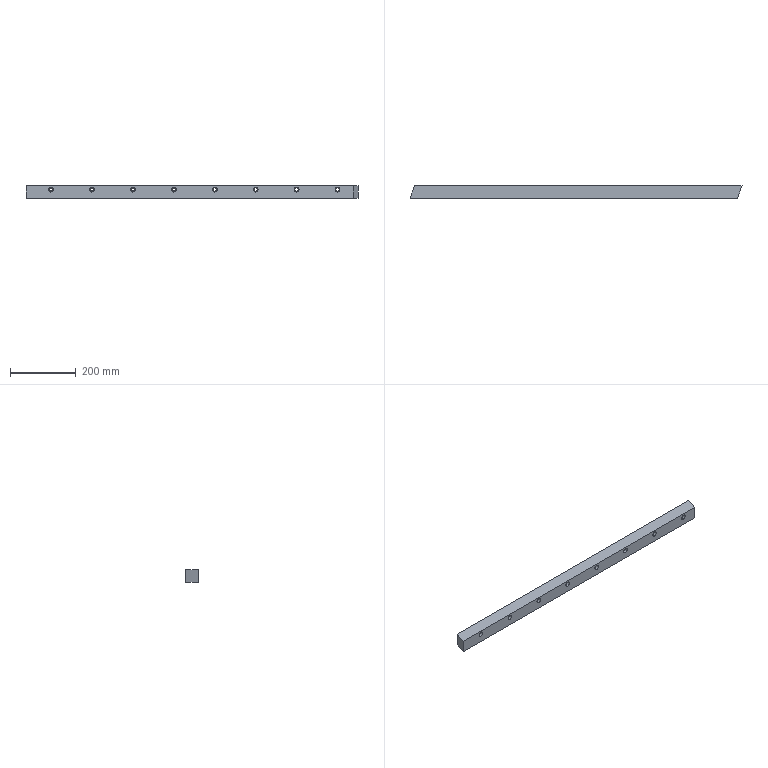Part | STEP file | MHH043910 | 1 solid | 46 faces | box 1014 x 39 x 39 mm | volume 1489427 mm3 | cylinder 32 | plane 14 | commonest cylinder face diameters 10 x16 15 x16
STEP:
#1=CARTESIAN_POINT('',(187.5,-30.,34.5));
#2=VERTEX_POINT('',#1);
#3=CARTESIAN_POINT('',(187.5,-30.,19.5));
#4=VERTEX_POINT('',#3);
#5=CARTESIAN_POINT('',(187.5,-30.,27.));
#6=DIRECTION('',(0.,-1.,0.));
#7=DIRECTION('',(0.,0.,-1.));
#8=AXIS2_PLACEMENT_3D('',#5,#6,#7);
#9=CIRCLE('',#8,7.5);
#10=EDGE_CURVE('',#2,#4,#9,.T.);
#11=ORIENTED_EDGE('',*,*,#10,.F.);
#12=CARTESIAN_POINT('',(187.5,-39.,34.5));
#13=VERTEX_POINT('',#12);
#14=CARTESIAN_POINT('',(187.5,-39.,34.5));
#15=DIRECTION('',(0.,-1.,0.));
#16=VECTOR('',#15,1000.);
#17=LINE('',#14,#16);
#18=EDGE_CURVE('',#2,#13,#17,.T.);
#19=ORIENTED_EDGE('',*,*,#18,.T.);
#20=CARTESIAN_POINT('',(187.5,-39.,19.5));
#21=VERTEX_POINT('',#20);
#22=CARTESIAN_POINT('',(187.5,-39.,27.));
#23=DIRECTION('',(0.,-1.,0.));
#24=DIRECTION('',(0.,0.,-1.));
#25=AXIS2_PLACEMENT_3D('',#22,#23,#24);
#26=CIRCLE('',#25,7.5);
#27=EDGE_CURVE('',#13,#21,#26,.T.);
#28=ORIENTED_EDGE('',*,*,#27,.T.);
#29=CARTESIAN_POINT('',(187.5,-39.,19.5));
#30=DIRECTION('',(0.,-1.,0.));
#31=VECTOR('',#30,1000.);
#32=LINE('',#29,#31);
#33=EDGE_CURVE('',#4,#21,#32,.T.);
#34=ORIENTED_EDGE('',*,*,#33,.F.);
#35=EDGE_LOOP('',(#11,#19,#28,#34));
#36=FACE_OUTER_BOUND('',#35,.T.);
#37=CARTESIAN_POINT('',(187.5,-39.,27.));
#38=DIRECTION('',(0.,-1.,0.));
#39=DIRECTION('',(0.,0.,-1.));
#40=AXIS2_PLACEMENT_3D('',#37,#38,#39);
#41=CYLINDRICAL_SURFACE('',#40,7.5);
#42=ADVANCED_FACE('',(#36),#41,.F.);
#43=CARTESIAN_POINT('',(187.5,0.,32.));
#44=VERTEX_POINT('',#43);
#45=CARTESIAN_POINT('',(187.5,0.,22.));
#46=VERTEX_POINT('',#45);
#47=CARTESIAN_POINT('',(187.5,0.,27.));
#48=DIRECTION('',(0.,-1.,0.));
#49=DIRECTION('',(0.,0.,-1.));
#50=AXIS2_PLACEMENT_3D('',#47,#48,#49);
#51=CIRCLE('',#50,5.);
#52=EDGE_CURVE('',#44,#46,#51,.T.);
#53=ORIENTED_EDGE('',*,*,#52,.F.);
#54=CARTESIAN_POINT('',(187.5,-30.,32.));
#55=VERTEX_POINT('',#54);
#56=CARTESIAN_POINT('',(187.5,-39.,32.));
#57=DIRECTION('',(0.,-1.,0.));
#58=VECTOR('',#57,1000.);
#59=LINE('',#56,#58);
#60=EDGE_CURVE('',#44,#55,#59,.T.);
#61=ORIENTED_EDGE('',*,*,#60,.T.);
#62=CARTESIAN_POINT('',(187.5,-30.,22.));
#63=VERTEX_POINT('',#62);
#64=CARTESIAN_POINT('',(187.5,-30.,27.));
#65=DIRECTION('',(0.,-1.,0.));
#66=DIRECTION('',(0.,0.,-1.));
#67=AXIS2_PLACEMENT_3D('',#64,#65,#66);
#68=CIRCLE('',#67,5.);
#69=EDGE_CURVE('',#55,#63,#68,.T.);
#70=ORIENTED_EDGE('',*,*,#69,.T.);
#71=CARTESIAN_POINT('',(187.5,-39.,22.));
#72=DIRECTION('',(0.,-1.,0.));
#73=VECTOR('',#72,1000.);
#74=LINE('',#71,#73);
#75=EDGE_CURVE('',#46,#63,#74,.T.);
#76=ORIENTED_EDGE('',*,*,#75,.F.);
#77=EDGE_LOOP('',(#53,#61,#70,#76));
#78=FACE_OUTER_BOUND('',#77,.T.);
#79=CARTESIAN_POINT('',(187.5,-39.,27.));
#80=DIRECTION('',(0.,-1.,0.));
#81=DIRECTION('',(0.,0.,-1.));
#82=AXIS2_PLACEMENT_3D('',#79,#80,#81);
#83=CYLINDRICAL_SURFACE('',#82,5.);
#84=ADVANCED_FACE('',(#78),#83,.F.);
#85=CARTESIAN_POINT('',(62.5,-30.,34.5));
#86=VERTEX_POINT('',#85);
#87=CARTESIAN_POINT('',(62.5,-30.,19.5));
#88=VERTEX_POINT('',#87);
#89=CARTESIAN_POINT('',(62.5,-30.,27.));
#90=DIRECTION('',(0.,-1.,0.));
#91=DIRECTION('',(0.,0.,-1.));
#92=AXIS2_PLACEMENT_3D('',#89,#90,#91);
#93=CIRCLE('',#92,7.5);
#94=EDGE_CURVE('',#86,#88,#93,.T.);
#95=ORIENTED_EDGE('',*,*,#94,.F.);
#96=CARTESIAN_POINT('',(62.5,-39.,34.5));
#97=VERTEX_POINT('',#96);
#98=CARTESIAN_POINT('',(62.5,-39.,34.5));
#99=DIRECTION('',(0.,-1.,0.));
#100=VECTOR('',#99,1000.);
#101=LINE('',#98,#100);
#102=EDGE_CURVE('',#86,#97,#101,.T.);
#103=ORIENTED_EDGE('',*,*,#102,.T.);
#104=CARTESIAN_POINT('',(62.5,-39.,19.5));
#105=VERTEX_POINT('',#104);
#106=CARTESIAN_POINT('',(62.5,-39.,27.));
#107=DIRECTION('',(0.,-1.,0.));
#108=DIRECTION('',(0.,0.,-1.));
#109=AXIS2_PLACEMENT_3D('',#106,#107,#108);
#110=CIRCLE('',#109,7.5);
#111=EDGE_CURVE('',#97,#105,#110,.T.);
#112=ORIENTED_EDGE('',*,*,#111,.T.);
#113=CARTESIAN_POINT('',(62.5,-39.,19.5));
#114=DIRECTION('',(0.,-1.,0.));
#115=VECTOR('',#114,1000.);
#116=LINE('',#113,#115);
#117=EDGE_CURVE('',#88,#105,#116,.T.);
#118=ORIENTED_EDGE('',*,*,#117,.F.);
#119=EDGE_LOOP('',(#95,#103,#112,#118));
#120=FACE_OUTER_BOUND('',#119,.T.);
#121=CARTESIAN_POINT('',(62.5,-39.,27.));
#122=DIRECTION('',(0.,-1.,0.));
#123=DIRECTION('',(0.,0.,-1.));
#124=AXIS2_PLACEMENT_3D('',#121,#122,#123);
#125=CYLINDRICAL_SURFACE('',#124,7.5);
#126=ADVANCED_FACE('',(#120),#125,.F.);
#127=CARTESIAN_POINT('',(62.5,0.,32.));
#128=VERTEX_POINT('',#127);
#129=CARTESIAN_POINT('',(62.5,0.,22.));
#130=VERTEX_POINT('',#129);
#131=CARTESIAN_POINT('',(62.5,0.,27.));
#132=DIRECTION('',(0.,-1.,0.));
#133=DIRECTION('',(0.,0.,-1.));
#134=AXIS2_PLACEMENT_3D('',#131,#132,#133);
#135=CIRCLE('',#134,5.);
#136=EDGE_CURVE('',#128,#130,#135,.T.);
#137=ORIENTED_EDGE('',*,*,#136,.F.);
#138=CARTESIAN_POINT('',(62.5,-30.,32.));
#139=VERTEX_POINT('',#138);
#140=CARTESIAN_POINT('',(62.5,-39.,32.));
#141=DIRECTION('',(0.,-1.,0.));
#142=VECTOR('',#141,1000.);
#143=LINE('',#140,#142);
#144=EDGE_CURVE('',#128,#139,#143,.T.);
#145=ORIENTED_EDGE('',*,*,#144,.T.);
#146=CARTESIAN_POINT('',(62.5,-30.,22.));
#147=VERTEX_POINT('',#146);
#148=CARTESIAN_POINT('',(62.5,-30.,27.));
#149=DIRECTION('',(0.,-1.,0.));
#150=DIRECTION('',(0.,0.,-1.));
#151=AXIS2_PLACEMENT_3D('',#148,#149,#150);
#152=CIRCLE('',#151,5.);
#153=EDGE_CURVE('',#139,#147,#152,.T.);
#154=ORIENTED_EDGE('',*,*,#153,.T.);
#155=CARTESIAN_POINT('',(62.5,-39.,22.));
#156=DIRECTION('',(0.,-1.,0.));
#157=VECTOR('',#156,1000.);
#158=LINE('',#155,#157);
#159=EDGE_CURVE('',#130,#147,#158,.T.);
#160=ORIENTED_EDGE('',*,*,#159,.F.);
#161=EDGE_LOOP('',(#137,#145,#154,#160));
#162=FACE_OUTER_BOUND('',#161,.T.);
#163=CARTESIAN_POINT('',(62.5,-39.,27.));
#164=DIRECTION('',(0.,-1.,0.));
#165=DIRECTION('',(0.,0.,-1.));
#166=AXIS2_PLACEMENT_3D('',#163,#164,#165);
#167=CYLINDRICAL_SURFACE('',#166,5.);
#168=ADVANCED_FACE('',(#162),#167,.F.);
#169=CARTESIAN_POINT('',(312.5,0.,32.));
#170=VERTEX_POINT('',#169);
#171=CARTESIAN_POINT('',(312.5,0.,22.));
#172=VERTEX_POINT('',#171);
#173=CARTESIAN_POINT('',(312.5,0.,27.));
#174=DIRECTION('',(0.,-1.,0.));
#175=DIRECTION('',(0.,0.,-1.));
#176=AXIS2_PLACEMENT_3D('',#173,#174,#175);
#177=CIRCLE('',#176,5.);
#178=EDGE_CURVE('',#170,#172,#177,.T.);
#179=ORIENTED_EDGE('',*,*,#178,.F.);
#180=CARTESIAN_POINT('',(312.5,-30.,32.));
#181=VERTEX_POINT('',#180);
#182=CARTESIAN_POINT('',(312.5,-39.,32.));
#183=DIRECTION('',(0.,-1.,0.));
#184=VECTOR('',#183,1000.);
#185=LINE('',#182,#184);
#186=EDGE_CURVE('',#170,#181,#185,.T.);
#187=ORIENTED_EDGE('',*,*,#186,.T.);
#188=CARTESIAN_POINT('',(312.5,-30.,22.));
#189=VERTEX_POINT('',#188);
#190=CARTESIAN_POINT('',(312.5,-30.,27.));
#191=DIRECTION('',(0.,-1.,0.));
#192=DIRECTION('',(0.,0.,-1.));
#193=AXIS2_PLACEMENT_3D('',#190,#191,#192);
#194=CIRCLE('',#193,5.);
#195=EDGE_CURVE('',#181,#189,#194,.T.);
#196=ORIENTED_EDGE('',*,*,#195,.T.);
#197=CARTESIAN_POINT('',(312.5,-39.,22.));
#198=DIRECTION('',(0.,-1.,0.));
#199=VECTOR('',#198,1000.);
#200=LINE('',#197,#199);
#201=EDGE_CURVE('',#172,#189,#200,.T.);
#202=ORIENTED_EDGE('',*,*,#201,.F.);
#203=EDGE_LOOP('',(#179,#187,#196,#202));
#204=FACE_OUTER_BOUND('',#203,.T.);
#205=CARTESIAN_POINT('',(312.5,-39.,27.));
#206=DIRECTION('',(0.,-1.,0.));
#207=DIRECTION('',(0.,0.,-1.));
#208=AXIS2_PLACEMENT_3D('',#205,#206,#207);
#209=CYLINDRICAL_SURFACE('',#208,5.);
#210=ADVANCED_FACE('',(#204),#209,.F.);
#211=CARTESIAN_POINT('',(312.5,-30.,34.5));
#212=VERTEX_POINT('',#211);
#213=CARTESIAN_POINT('',(312.5,-30.,19.5));
#214=VERTEX_POINT('',#213);
#215=CARTESIAN_POINT('',(312.5,-30.,27.));
#216=DIRECTION('',(0.,-1.,0.));
#217=DIRECTION('',(0.,0.,-1.));
#218=AXIS2_PLACEMENT_3D('',#215,#216,#217);
#219=CIRCLE('',#218,7.5);
#220=EDGE_CURVE('',#212,#214,#219,.T.);
#221=ORIENTED_EDGE('',*,*,#220,.F.);
#222=CARTESIAN_POINT('',(312.5,-39.,34.5));
#223=VERTEX_POINT('',#222);
#224=CARTESIAN_POINT('',(312.5,-39.,34.5));
#225=DIRECTION('',(0.,-1.,0.));
#226=VECTOR('',#225,1000.);
#227=LINE('',#224,#226);
#228=EDGE_CURVE('',#212,#223,#227,.T.);
#229=ORIENTED_EDGE('',*,*,#228,.T.);
#230=CARTESIAN_POINT('',(312.5,-39.,19.5));
#231=VERTEX_POINT('',#230);
#232=CARTESIAN_POINT('',(312.5,-39.,27.));
#233=DIRECTION('',(0.,-1.,0.));
#234=DIRECTION('',(0.,0.,-1.));
#235=AXIS2_PLACEMENT_3D('',#232,#233,#234);
#236=CIRCLE('',#235,7.5);
#237=EDGE_CURVE('',#223,#231,#236,.T.);
#238=ORIENTED_EDGE('',*,*,#237,.T.);
#239=CARTESIAN_POINT('',(312.5,-39.,19.5));
#240=DIRECTION('',(0.,-1.,0.));
#241=VECTOR('',#240,1000.);
#242=LINE('',#239,#241);
#243=EDGE_CURVE('',#214,#231,#242,.T.);
#244=ORIENTED_EDGE('',*,*,#243,.F.);
#245=EDGE_LOOP('',(#221,#229,#238,#244));
#246=FACE_OUTER_BOUND('',#245,.T.);
#247=CARTESIAN_POINT('',(312.5,-39.,27.));
#248=DIRECTION('',(0.,-1.,0.));
#249=DIRECTION('',(0.,0.,-1.));
#250=AXIS2_PLACEMENT_3D('',#247,#248,#249);
#251=CYLINDRICAL_SURFACE('',#250,7.5);
#252=ADVANCED_FACE('',(#246),#251,.F.);
#253=CARTESIAN_POINT('',(437.5,0.,32.));
#254=VERTEX_POINT('',#253);
#255=CARTESIAN_POINT('',(437.5,0.,22.));
#256=VERTEX_POINT('',#255);
#257=CARTESIAN_POINT('',(437.5,0.,27.));
#258=DIRECTION('',(0.,-1.,0.));
#259=DIRECTION('',(0.,0.,-1.));
#260=AXIS2_PLACEMENT_3D('',#257,#258,#259);
#261=CIRCLE('',#260,5.);
#262=EDGE_CURVE('',#254,#256,#261,.T.);
#263=ORIENTED_EDGE('',*,*,#262,.F.);
#264=CARTESIAN_POINT('',(437.5,-30.,32.));
#265=VERTEX_POINT('',#264);
#266=CARTESIAN_POINT('',(437.5,-39.,32.));
#267=DIRECTION('',(0.,-1.,0.));
#268=VECTOR('',#267,1000.);
#269=LINE('',#266,#268);
#270=EDGE_CURVE('',#254,#265,#269,.T.);
#271=ORIENTED_EDGE('',*,*,#270,.T.);
#272=CARTESIAN_POINT('',(437.5,-30.,22.));
#273=VERTEX_POINT('',#272);
#274=CARTESIAN_POINT('',(437.5,-30.,27.));
#275=DIRECTION('',(0.,-1.,0.));
#276=DIRECTION('',(0.,0.,-1.));
#277=AXIS2_PLACEMENT_3D('',#274,#275,#276);
#278=CIRCLE('',#277,5.);
#279=EDGE_CURVE('',#265,#273,#278,.T.);
#280=ORIENTED_EDGE('',*,*,#279,.T.);
#281=CARTESIAN_POINT('',(437.5,-39.,22.));
#282=DIRECTION('',(0.,-1.,0.));
#283=VECTOR('',#282,1000.);
#284=LINE('',#281,#283);
#285=EDGE_CURVE('',#256,#273,#284,.T.);
#286=ORIENTED_EDGE('',*,*,#285,.F.);
#287=EDGE_LOOP('',(#263,#271,#280,#286));
#288=FACE_OUTER_BOUND('',#287,.T.);
#289=CARTESIAN_POINT('',(437.5,-39.,27.));
#290=DIRECTION('',(0.,-1.,0.));
#291=DIRECTION('',(0.,0.,-1.));
#292=AXIS2_PLACEMENT_3D('',#289,#290,#291);
#293=CYLINDRICAL_SURFACE('',#292,5.);
#294=ADVANCED_FACE('',(#288),#293,.F.);
#295=CARTESIAN_POINT('',(437.5,-30.,34.5));
#296=VERTEX_POINT('',#295);
#297=CARTESIAN_POINT('',(437.5,-30.,19.5));
#298=VERTEX_POINT('',#297);
#299=CARTESIAN_POINT('',(437.5,-30.,27.));
#300=DIRECTION('',(0.,-1.,0.));
#301=DIRECTION('',(0.,0.,-1.));
#302=AXIS2_PLACEMENT_3D('',#299,#300,#301);
#303=CIRCLE('',#302,7.5);
#304=EDGE_CURVE('',#296,#298,#303,.T.);
#305=ORIENTED_EDGE('',*,*,#304,.F.);
#306=CARTESIAN_POINT('',(437.5,-39.,34.5));
#307=VERTEX_POINT('',#306);
#308=CARTESIAN_POINT('',(437.5,-39.,34.5));
#309=DIRECTION('',(0.,-1.,0.));
#310=VECTOR('',#309,1000.);
#311=LINE('',#308,#310);
#312=EDGE_CURVE('',#296,#307,#311,.T.);
#313=ORIENTED_EDGE('',*,*,#312,.T.);
#314=CARTESIAN_POINT('',(437.5,-39.,19.5));
#315=VERTEX_POINT('',#314);
#316=CARTESIAN_POINT('',(437.5,-39.,27.));
#317=DIRECTION('',(0.,-1.,0.));
#318=DIRECTION('',(0.,0.,-1.));
#319=AXIS2_PLACEMENT_3D('',#316,#317,#318);
#320=CIRCLE('',#319,7.5);
#321=EDGE_CURVE('',#307,#315,#320,.T.);
#322=ORIENTED_EDGE('',*,*,#321,.T.);
#323=CARTESIAN_POINT('',(437.5,-39.,19.5));
#324=DIRECTION('',(0.,-1.,0.));
#325=VECTOR('',#324,1000.);
#326=LINE('',#323,#325);
#327=EDGE_CURVE('',#298,#315,#326,.T.);
#328=ORIENTED_EDGE('',*,*,#327,.F.);
#329=EDGE_LOOP('',(#305,#313,#322,#328));
#330=FACE_OUTER_BOUND('',#329,.T.);
#331=CARTESIAN_POINT('',(437.5,-39.,27.));
#332=DIRECTION('',(0.,-1.,0.));
#333=DIRECTION('',(0.,0.,-1.));
#334=AXIS2_PLACEMENT_3D('',#331,#332,#333);
#335=CYLINDRICAL_SURFACE('',#334,7.5);
#336=ADVANCED_FACE('',(#330),#335,.F.);
#337=CARTESIAN_POINT('',(562.5,0.,32.));
#338=VERTEX_POINT('',#337);
#339=CARTESIAN_POINT('',(562.5,0.,22.));
#340=VERTEX_POINT('',#339);
#341=CARTESIAN_POINT('',(562.5,0.,27.));
#342=DIRECTION('',(0.,-1.,0.));
#343=DIRECTION('',(0.,0.,-1.));
#344=AXIS2_PLACEMENT_3D('',#341,#342,#343);
#345=CIRCLE('',#344,5.);
#346=EDGE_CURVE('',#338,#340,#345,.T.);
#347=ORIENTED_EDGE('',*,*,#346,.F.);
#348=CARTESIAN_POINT('',(562.5,-30.,32.));
#349=VERTEX_POINT('',#348);
#350=CARTESIAN_POINT('',(562.5,-39.,32.));
#351=DIRECTION('',(0.,-1.,0.));
#352=VECTOR('',#351,1000.);
#353=LINE('',#350,#352);
#354=EDGE_CURVE('',#338,#349,#353,.T.);
#355=ORIENTED_EDGE('',*,*,#354,.T.);
#356=CARTESIAN_POINT('',(562.5,-30.,22.));
#357=VERTEX_POINT('',#356);
#358=CARTESIAN_POINT('',(562.5,-30.,27.));
#359=DIRECTION('',(0.,-1.,0.));
#360=DIRECTION('',(0.,0.,-1.));
#361=AXIS2_PLACEMENT_3D('',#358,#359,#360);
#362=CIRCLE('',#361,5.);
#363=EDGE_CURVE('',#349,#357,#362,.T.);
#364=ORIENTED_EDGE('',*,*,#363,.T.);
#365=CARTESIAN_POINT('',(562.5,-39.,22.));
#366=DIRECTION('',(0.,-1.,0.));
#367=VECTOR('',#366,1000.);
#368=LINE('',#365,#367);
#369=EDGE_CURVE('',#340,#357,#368,.T.);
#370=ORIENTED_EDGE('',*,*,#369,.F.);
#371=EDGE_LOOP('',(#347,#355,#364,#370));
#372=FACE_OUTER_BOUND('',#371,.T.);
#373=CARTESIAN_POINT('',(562.5,-39.,27.));
#374=DIRECTION('',(0.,-1.,0.));
#375=DIRECTION('',(0.,0.,-1.));
#376=AXIS2_PLACEMENT_3D('',#373,#374,#375);
#377=CYLINDRICAL_SURFACE('',#376,5.);
#378=ADVANCED_FACE('',(#372),#377,.F.);
#379=CARTESIAN_POINT('',(562.5,-30.,34.5));
#380=VERTEX_POINT('',#379);
#381=CARTESIAN_POINT('',(562.5,-30.,19.5));
#382=VERTEX_POINT('',#381);
#383=CARTESIAN_POINT('',(562.5,-30.,27.));
#384=DIRECTION('',(0.,-1.,0.));
#385=DIRECTION('',(0.,0.,-1.));
#386=AXIS2_PLACEMENT_3D('',#383,#384,#385);
#387=CIRCLE('',#386,7.5);
#388=EDGE_CURVE('',#380,#382,#387,.T.);
#389=ORIENTED_EDGE('',*,*,#388,.F.);
#390=CARTESIAN_POINT('',(562.5,-39.,34.5));
#391=VERTEX_POINT('',#390);
#392=CARTESIAN_POINT('',(562.5,-39.,34.5));
#393=DIRECTION('',(0.,-1.,0.));
#394=VECTOR('',#393,1000.);
#395=LINE('',#392,#394);
#396=EDGE_CURVE('',#380,#391,#395,.T.);
#397=ORIENTED_EDGE('',*,*,#396,.T.);
#398=CARTESIAN_POINT('',(562.5,-39.,19.5));
#399=VERTEX_POINT('',#398);
#400=CARTESIAN_POINT('',(562.5,-39.,27.));
#401=DIRECTION('',(0.,-1.,0.));
#402=DIRECTION('',(0.,0.,-1.));
#403=AXIS2_PLACEMENT_3D('',#400,#401,#402);
#404=CIRCLE('',#403,7.5);
#405=EDGE_CURVE('',#391,#399,#404,.T.);
#406=ORIENTED_EDGE('',*,*,#405,.T.);
#407=CARTESIAN_POINT('',(562.5,-39.,19.5));
#408=DIRECTION('',(0.,-1.,0.));
#409=VECTOR('',#408,1000.);
#410=LINE('',#407,#409);
#411=EDGE_CURVE('',#382,#399,#410,.T.);
#412=ORIENTED_EDGE('',*,*,#411,.F.);
#413=EDGE_LOOP('',(#389,#397,#406,#412));
#414=FACE_OUTER_BOUND('',#413,.T.);
#415=CARTESIAN_POINT('',(562.5,-39.,27.));
#416=DIRECTION('',(0.,-1.,0.));
#417=DIRECTION('',(0.,0.,-1.));
#418=AXIS2_PLACEMENT_3D('',#415,#416,#417);
#419=CYLINDRICAL_SURFACE('',#418,7.5);
#420=ADVANCED_FACE('',(#414),#419,.F.);
#421=CARTESIAN_POINT('',(687.5,0.,32.));
#422=VERTEX_POINT('',#421);
#423=CARTESIAN_POINT('',(687.5,0.,22.));
#424=VERTEX_POINT('',#423);
#425=CARTESIAN_POINT('',(687.5,0.,27.));
#426=DIRECTION('',(0.,-1.,0.));
#427=DIRECTION('',(0.,0.,-1.));
#428=AXIS2_PLACEMENT_3D('',#425,#426,#427);
#429=CIRCLE('',#428,5.);
#430=EDGE_CURVE('',#422,#424,#429,.T.);
#431=ORIENTED_EDGE('',*,*,#430,.F.);
#432=CARTESIAN_POINT('',(687.5,-30.,32.));
#433=VERTEX_POINT('',#432);
#434=CARTESIAN_POINT('',(687.5,-39.,32.));
#435=DIRECTION('',(0.,-1.,0.));
#436=VECTOR('',#435,1000.);
#437=LINE('',#434,#436);
#438=EDGE_CURVE('',#422,#433,#437,.T.);
#439=ORIENTED_EDGE('',*,*,#438,.T.);
#440=CARTESIAN_POINT('',(687.5,-30.,22.));
#441=VERTEX_POINT('',#440);
#442=CARTESIAN_POINT('',(687.5,-30.,27.));
#443=DIRECTION('',(0.,-1.,0.));
#444=DIRECTION('',(0.,0.,-1.));
#445=AXIS2_PLACEMENT_3D('',#442,#443,#444);
#446=CIRCLE('',#445,5.);
#447=EDGE_CURVE('',#433,#441,#446,.T.);
#448=ORIENTED_EDGE('',*,*,#447,.T.);
#449=CARTESIAN_POINT('',(687.5,-39.,22.));
#450=DIRECTION('',(0.,-1.,0.));
#451=VECTOR('',#450,1000.);
#452=LINE('',#449,#451);
#453=EDGE_CURVE('',#424,#441,#452,.T.);
#454=ORIENTED_EDGE('',*,*,#453,.F.);
#455=EDGE_LOOP('',(#431,#439,#448,#454));
#456=FACE_OUTER_BOUND('',#455,.T.);
#457=CARTESIAN_POINT('',(687.5,-39.,27.));
#458=DIRECTION('',(0.,-1.,0.));
#459=DIRECTION('',(0.,0.,-1.));
#460=AXIS2_PLACEMENT_3D('',#457,#458,#459);
#461=CYLINDRICAL_SURFACE('',#460,5.);
#462=ADVANCED_FACE('',(#456),#461,.F.);
#463=CARTESIAN_POINT('',(687.5,-30.,34.5));
#464=VERTEX_POINT('',#463);
#465=CARTESIAN_POINT('',(687.5,-30.,19.5));
#466=VERTEX_POINT('',#465);
#467=CARTESIAN_POINT('',(687.5,-30.,27.));
#468=DIRECTION('',(0.,-1.,0.));
#469=DIRECTION('',(0.,0.,-1.));
#470=AXIS2_PLACEMENT_3D('',#467,#468,#469);
#471=CIRCLE('',#470,7.5);
#472=EDGE_CURVE('',#464,#466,#471,.T.);
#473=ORIENTED_EDGE('',*,*,#472,.F.);
#474=CARTESIAN_POINT('',(687.5,-39.,34.5));
#475=VERTEX_POINT('',#474);
#476=CARTESIAN_POINT('',(687.5,-39.,34.5));
#477=DIRECTION('',(0.,-1.,0.));
#478=VECTOR('',#477,1000.);
#479=LINE('',#476,#478);
#480=EDGE_CURVE('',#464,#475,#479,.T.);
#481=ORIENTED_EDGE('',*,*,#480,.T.);
#482=CARTESIAN_POINT('',(687.5,-39.,19.5));
#483=VERTEX_POINT('',#482);
#484=CARTESIAN_POINT('',(687.5,-39.,27.));
#485=DIRECTION('',(0.,-1.,0.));
#486=DIRECTION('',(0.,0.,-1.));
#487=AXIS2_PLACEMENT_3D('',#484,#485,#486);
#488=CIRCLE('',#487,7.5);
#489=EDGE_CURVE('',#475,#483,#488,.T.);
#490=ORIENTED_EDGE('',*,*,#489,.T.);
#491=CARTESIAN_POINT('',(687.5,-39.,19.5));
#492=DIRECTION('',(0.,-1.,0.));
#493=VECTOR('',#492,1000.);
#494=LINE('',#491,#493);
#495=EDGE_CURVE('',#466,#483,#494,.T.);
#496=ORIENTED_EDGE('',*,*,#495,.F.);
#497=EDGE_LOOP('',(#473,#481,#490,#496));
#498=FACE_OUTER_BOUND('',#497,.T.);
#499=CARTESIAN_POINT('',(687.5,-39.,27.));
#500=DIRECTION('',(0.,-1.,0.));
#501=DIRECTION('',(0.,0.,-1.));
#502=AXIS2_PLACEMENT_3D('',#499,#500,#501);
#503=CYLINDRICAL_SURFACE('',#502,7.5);
#504=ADVANCED_FACE('',(#498),#503,.F.);
#505=CARTESIAN_POINT('',(812.5,0.,32.));
#506=VERTEX_POINT('',#505);
#507=CARTESIAN_POINT('',(812.5,0.,22.));
#508=VERTEX_POINT('',#507);
#509=CARTESIAN_POINT('',(812.5,0.,27.));
#510=DIRECTION('',(0.,-1.,0.));
#511=DIRECTION('',(0.,0.,-1.));
#512=AXIS2_PLACEMENT_3D('',#509,#510,#511);
#513=CIRCLE('',#512,5.);
#514=EDGE_CURVE('',#506,#508,#513,.T.);
#515=ORIENTED_EDGE('',*,*,#514,.F.);
#516=CARTESIAN_POINT('',(812.5,-30.,32.));
#517=VERTEX_POINT('',#516);
#518=CARTESIAN_POINT('',(812.5,-39.,32.));
#519=DIRECTION('',(0.,-1.,0.));
#520=VECTOR('',#519,1000.);
#521=LINE('',#518,#520);
#522=EDGE_CURVE('',#506,#517,#521,.T.);
#523=ORIENTED_EDGE('',*,*,#522,.T.);
#524=CARTESIAN_POINT('',(812.5,-30.,22.));
#525=VERTEX_POINT('',#524);
#526=CARTESIAN_POINT('',(812.5,-30.,27.));
#527=DIRECTION('',(0.,-1.,0.));
#528=DIRECTION('',(0.,0.,-1.));
#529=AXIS2_PLACEMENT_3D('',#526,#527,#528);
#530=CIRCLE('',#529,5.);
#531=EDGE_CURVE('',#517,#525,#530,.T.);
#532=ORIENTED_EDGE('',*,*,#531,.T.);
#533=CARTESIAN_POINT('',(812.5,-39.,22.));
#534=DIRECTION('',(0.,-1.,0.));
#535=VECTOR('',#534,1000.);
#536=LINE('',#533,#535);
#537=EDGE_CURVE('',#508,#525,#536,.T.);
#538=ORIENTED_EDGE('',*,*,#537,.F.);
#539=EDGE_LOOP('',(#515,#523,#532,#538));
#540=FACE_OUTER_BOUND('',#539,.T.);
#541=CARTESIAN_POINT('',(812.5,-39.,27.));
#542=DIRECTION('',(0.,-1.,0.));
#543=DIRECTION('',(0.,0.,-1.));
#544=AXIS2_PLACEMENT_3D('',#541,#542,#543);
#545=CYLINDRICAL_SURFACE('',#544,5.);
#546=ADVANCED_FACE('',(#540),#545,.F.);
#547=CARTESIAN_POINT('',(812.5,-30.,34.5));
#548=VERTEX_POINT('',#547);
#549=CARTESIAN_POINT('',(812.5,-30.,19.5));
#550=VERTEX_POINT('',#549);
#551=CARTESIAN_POINT('',(812.5,-30.,27.));
#552=DIRECTION('',(0.,-1.,0.));
#553=DIRECTION('',(0.,0.,-1.));
#554=AXIS2_PLACEMENT_3D('',#551,#552,#553);
#555=CIRCLE('',#554,7.5);
#556=EDGE_CURVE('',#548,#550,#555,.T.);
#557=ORIENTED_EDGE('',*,*,#556,.F.);
#558=CARTESIAN_POINT('',(812.5,-39.,34.5));
#559=VERTEX_POINT('',#558);
#560=CARTESIAN_POINT('',(812.5,-39.,34.5));
#561=DIRECTION('',(0.,-1.,0.));
#562=VECTOR('',#561,1000.);
#563=LINE('',#560,#562);
#564=EDGE_CURVE('',#548,#559,#563,.T.);
#565=ORIENTED_EDGE('',*,*,#564,.T.);
#566=CARTESIAN_POINT('',(812.5,-39.,19.5));
#567=VERTEX_POINT('',#566);
#568=CARTESIAN_POINT('',(812.5,-39.,27.));
#569=DIRECTION('',(0.,-1.,0.));
#570=DIRECTION('',(0.,0.,-1.));
#571=AXIS2_PLACEMENT_3D('',#568,#569,#570);
#572=CIRCLE('',#571,7.5);
#573=EDGE_CURVE('',#559,#567,#572,.T.);
#574=ORIENTED_EDGE('',*,*,#573,.T.);
#575=CARTESIAN_POINT('',(812.5,-39.,19.5));
#576=DIRECTION('',(0.,-1.,0.));
#577=VECTOR('',#576,1000.);
#578=LINE('',#575,#577);
#579=EDGE_CURVE('',#550,#567,#578,.T.);
#580=ORIENTED_EDGE('',*,*,#579,.F.);
#581=EDGE_LOOP('',(#557,#565,#574,#580));
#582=FACE_OUTER_BOUND('',#581,.T.);
#583=CARTESIAN_POINT('',(812.5,-39.,27.));
#584=DIRECTION('',(0.,-1.,0.));
#585=DIRECTION('',(0.,0.,-1.));
#586=AXIS2_PLACEMENT_3D('',#583,#584,#585);
#587=CYLINDRICAL_SURFACE('',#586,7.5);
#588=ADVANCED_FACE('',(#582),#587,.F.);
#589=CARTESIAN_POINT('',(937.5,0.,32.));
#590=VERTEX_POINT('',#589);
#591=CARTESIAN_POINT('',(937.5,0.,22.));
#592=VERTEX_POINT('',#591);
#593=CARTESIAN_POINT('',(937.5,0.,27.));
#594=DIRECTION('',(0.,-1.,0.));
#595=DIRECTION('',(0.,0.,-1.));
#596=AXIS2_PLACEMENT_3D('',#593,#594,#595);
#597=CIRCLE('',#596,5.);
#598=EDGE_CURVE('',#590,#592,#597,.T.);
#599=ORIENTED_EDGE('',*,*,#598,.F.);
#600=CARTESIAN_POINT('',(937.5,-30.,32.));
#601=VERTEX_POINT('',#600);
#602=CARTESIAN_POINT('',(937.5,-39.,32.));
#603=DIRECTION('',(0.,-1.,0.));
#604=VECTOR('',#603,1000.);
#605=LINE('',#602,#604);
#606=EDGE_CURVE('',#590,#601,#605,.T.);
#607=ORIENTED_EDGE('',*,*,#606,.T.);
#608=CARTESIAN_POINT('',(937.5,-30.,22.));
#609=VERTEX_POINT('',#608);
#610=CARTESIAN_POINT('',(937.5,-30.,27.));
#611=DIRECTION('',(0.,-1.,0.));
#612=DIRECTION('',(0.,0.,-1.));
#613=AXIS2_PLACEMENT_3D('',#610,#611,#612);
#614=CIRCLE('',#613,5.);
#615=EDGE_CURVE('',#601,#609,#614,.T.);
#616=ORIENTED_EDGE('',*,*,#615,.T.);
#617=CARTESIAN_POINT('',(937.5,-39.,22.));
#618=DIRECTION('',(0.,-1.,0.));
#619=VECTOR('',#618,1000.);
#620=LINE('',#617,#619);
#621=EDGE_CURVE('',#592,#609,#620,.T.);
#622=ORIENTED_EDGE('',*,*,#621,.F.);
#623=EDGE_LOOP('',(#599,#607,#616,#622));
#624=FACE_OUTER_BOUND('',#623,.T.);
#625=CARTESIAN_POINT('',(937.5,-39.,27.));
#626=DIRECTION('',(0.,-1.,0.));
#627=DIRECTION('',(0.,0.,-1.));
#628=AXIS2_PLACEMENT_3D('',#625,#626,#627);
#629=CYLINDRICAL_SURFACE('',#628,5.);
#630=ADVANCED_FACE('',(#624),#629,.F.);
#631=CARTESIAN_POINT('',(937.5,-30.,34.5));
#632=VERTEX_POINT('',#631);
#633=CARTESIAN_POINT('',(937.5,-30.,19.5));
#634=VERTEX_POINT('',#633);
#635=CARTESIAN_POINT('',(937.5,-30.,27.));
#636=DIRECTION('',(0.,-1.,0.));
#637=DIRECTION('',(0.,0.,-1.));
#638=AXIS2_PLACEMENT_3D('',#635,#636,#637);
#639=CIRCLE('',#638,7.5);
#640=EDGE_CURVE('',#632,#634,#639,.T.);
#641=ORIENTED_EDGE('',*,*,#640,.F.);
#642=CARTESIAN_POINT('',(937.5,-39.,34.5));
#643=VERTEX_POINT('',#642);
#644=CARTESIAN_POINT('',(937.5,-39.,34.5));
#645=DIRECTION('',(0.,-1.,0.));
#646=VECTOR('',#645,1000.);
#647=LINE('',#644,#646);
#648=EDGE_CURVE('',#632,#643,#647,.T.);
#649=ORIENTED_EDGE('',*,*,#648,.T.);
#650=CARTESIAN_POINT('',(937.5,-39.,19.5));
#651=VERTEX_POINT('',#650);
#652=CARTESIAN_POINT('',(937.5,-39.,27.));
#653=DIRECTION('',(0.,-1.,0.));
#654=DIRECTION('',(0.,0.,-1.));
#655=AXIS2_PLACEMENT_3D('',#652,#653,#654);
#656=CIRCLE('',#655,7.5);
#657=EDGE_CURVE('',#643,#651,#656,.T.);
#658=ORIENTED_EDGE('',*,*,#657,.T.);
#659=CARTESIAN_POINT('',(937.5,-39.,19.5));
#660=DIRECTION('',(0.,-1.,0.));
#661=VECTOR('',#660,1000.);
#662=LINE('',#659,#661);
#663=EDGE_CURVE('',#634,#651,#662,.T.);
#664=ORIENTED_EDGE('',*,*,#663,.F.);
#665=EDGE_LOOP('',(#641,#649,#658,#664));
#666=FACE_OUTER_BOUND('',#665,.T.);
#667=CARTESIAN_POINT('',(937.5,-39.,27.));
#668=DIRECTION('',(0.,-1.,0.));
#669=DIRECTION('',(0.,0.,-1.));
#670=AXIS2_PLACEMENT_3D('',#667,#668,#669);
#671=CYLINDRICAL_SURFACE('',#670,7.5);
#672=ADVANCED_FACE('',(#666),#671,.F.);
#673=ORIENTED_EDGE('',*,*,#648,.F.);
#674=CARTESIAN_POINT('',(937.5,-30.,27.));
#675=DIRECTION('',(0.,-1.,0.));
#676=DIRECTION('',(0.,0.,-1.));
#677=AXIS2_PLACEMENT_3D('',#674,#675,#676);
#678=CIRCLE('',#677,7.5);
#679=EDGE_CURVE('',#634,#632,#678,.T.);
#680=ORIENTED_EDGE('',*,*,#679,.F.);
#681=ORIENTED_EDGE('',*,*,#663,.T.);
#682=CARTESIAN_POINT('',(937.5,-39.,27.));
#683=DIRECTION('',(0.,-1.,0.));
#684=DIRECTION('',(0.,0.,-1.));
#685=AXIS2_PLACEMENT_3D('',#682,#683,#684);
#686=CIRCLE('',#685,7.5);
#687=EDGE_CURVE('',#651,#643,#686,.T.);
#688=ORIENTED_EDGE('',*,*,#687,.T.);
#689=EDGE_LOOP('',(#673,#680,#681,#688));
#690=FACE_OUTER_BOUND('',#689,.T.);
#691=CARTESIAN_POINT('',(937.5,-39.,27.));
#692=DIRECTION('',(0.,-1.,0.));
#693=DIRECTION('',(0.,0.,-1.));
#694=AXIS2_PLACEMENT_3D('',#691,#692,#693);
#695=CYLINDRICAL_SURFACE('',#694,7.5);
#696=ADVANCED_FACE('',(#690),#695,.F.);
#697=CARTESIAN_POINT('',(937.5,-30.,27.));
#698=DIRECTION('',(0.,-1.,0.));
#699=DIRECTION('',(0.,0.,-1.));
#700=AXIS2_PLACEMENT_3D('',#697,#698,#699);
#701=CIRCLE('',#700,5.);
#702=EDGE_CURVE('',#609,#601,#701,.T.);
#703=ORIENTED_EDGE('',*,*,#702,.F.);
#704=ORIENTED_EDGE('',*,*,#615,.F.);
#705=EDGE_LOOP('',(#703,#704));
#706=FACE_BOUND('',#705,.T.);
#707=ORIENTED_EDGE('',*,*,#679,.T.);
#708=ORIENTED_EDGE('',*,*,#640,.T.);
#709=EDGE_LOOP('',(#707,#708));
#710=FACE_OUTER_BOUND('',#709,.T.);
#711=CARTESIAN_POINT('',(942.5,-30.,27.));
#712=DIRECTION('',(0.,1.,0.));
#713=DIRECTION('',(0.,0.,1.));
#714=AXIS2_PLACEMENT_3D('',#711,#712,#713);
#715=PLANE('',#714);
#716=ADVANCED_FACE('',(#706,#710),#715,.F.);
#717=ORIENTED_EDGE('',*,*,#606,.F.);
#718=CARTESIAN_POINT('',(937.5,0.,27.));
#719=DIRECTION('',(0.,-1.,0.));
#720=DIRECTION('',(0.,0.,-1.));
#721=AXIS2_PLACEMENT_3D('',#718,#719,#720);
#722=CIRCLE('',#721,5.);
#723=EDGE_CURVE('',#592,#590,#722,.T.);
#724=ORIENTED_EDGE('',*,*,#723,.F.);
#725=ORIENTED_EDGE('',*,*,#621,.T.);
#726=ORIENTED_EDGE('',*,*,#702,.T.);
#727=EDGE_LOOP('',(#717,#724,#725,#726));
#728=FACE_OUTER_BOUND('',#727,.T.);
#729=CARTESIAN_POINT('',(937.5,-39.,27.));
#730=DIRECTION('',(0.,-1.,0.));
#731=DIRECTION('',(0.,0.,-1.));
#732=AXIS2_PLACEMENT_3D('',#729,#730,#731);
#733=CYLINDRICAL_SURFACE('',#732,5.);
#734=ADVANCED_FACE('',(#728),#733,.F.);
#735=ORIENTED_EDGE('',*,*,#564,.F.);
#736=CARTESIAN_POINT('',(812.5,-30.,27.));
#737=DIRECTION('',(0.,-1.,0.));
#738=DIRECTION('',(0.,0.,-1.));
#739=AXIS2_PLACEMENT_3D('',#736,#737,#738);
#740=CIRCLE('',#739,7.5);
#741=EDGE_CURVE('',#550,#548,#740,.T.);
#742=ORIENTED_EDGE('',*,*,#741,.F.);
#743=ORIENTED_EDGE('',*,*,#579,.T.);
#744=CARTESIAN_POINT('',(812.5,-39.,27.));
#745=DIRECTION('',(0.,-1.,0.));
#746=DIRECTION('',(0.,0.,-1.));
#747=AXIS2_PLACEMENT_3D('',#744,#745,#746);
#748=CIRCLE('',#747,7.5);
#749=EDGE_CURVE('',#567,#559,#748,.T.);
#750=ORIENTED_EDGE('',*,*,#749,.T.);
#751=EDGE_LOOP('',(#735,#742,#743,#750));
#752=FACE_OUTER_BOUND('',#751,.T.);
#753=CARTESIAN_POINT('',(812.5,-39.,27.));
#754=DIRECTION('',(0.,-1.,0.));
#755=DIRECTION('',(0.,0.,-1.));
#756=AXIS2_PLACEMENT_3D('',#753,#754,#755);
#757=CYLINDRICAL_SURFACE('',#756,7.5);
#758=ADVANCED_FACE('',(#752),#757,.F.);
#759=CARTESIAN_POINT('',(812.5,-30.,27.));
#760=DIRECTION('',(0.,-1.,0.));
#761=DIRECTION('',(0.,0.,-1.));
#762=AXIS2_PLACEMENT_3D('',#759,#760,#761);
#763=CIRCLE('',#762,5.);
#764=EDGE_CURVE('',#525,#517,#763,.T.);
#765=ORIENTED_EDGE('',*,*,#764,.F.);
#766=ORIENTED_EDGE('',*,*,#531,.F.);
#767=EDGE_LOOP('',(#765,#766));
#768=FACE_BOUND('',#767,.T.);
#769=ORIENTED_EDGE('',*,*,#741,.T.);
#770=ORIENTED_EDGE('',*,*,#556,.T.);
#771=EDGE_LOOP('',(#769,#770));
#772=FACE_OUTER_BOUND('',#771,.T.);
#773=CARTESIAN_POINT('',(817.5,-30.,27.));
#774=DIRECTION('',(0.,1.,0.));
#775=DIRECTION('',(0.,0.,1.));
#776=AXIS2_PLACEMENT_3D('',#773,#774,#775);
#777=PLANE('',#776);
#778=ADVANCED_FACE('',(#768,#772),#777,.F.);
#779=ORIENTED_EDGE('',*,*,#522,.F.);
#780=CARTESIAN_POINT('',(812.5,0.,27.));
#781=DIRECTION('',(0.,-1.,0.));
#782=DIRECTION('',(0.,0.,-1.));
#783=AXIS2_PLACEMENT_3D('',#780,#781,#782);
#784=CIRCLE('',#783,5.);
#785=EDGE_CURVE('',#508,#506,#784,.T.);
#786=ORIENTED_EDGE('',*,*,#785,.F.);
#787=ORIENTED_EDGE('',*,*,#537,.T.);
#788=ORIENTED_EDGE('',*,*,#764,.T.);
#789=EDGE_LOOP('',(#779,#786,#787,#788));
#790=FACE_OUTER_BOUND('',#789,.T.);
#791=CARTESIAN_POINT('',(812.5,-39.,27.));
#792=DIRECTION('',(0.,-1.,0.));
#793=DIRECTION('',(0.,0.,-1.));
#794=AXIS2_PLACEMENT_3D('',#791,#792,#793);
#795=CYLINDRICAL_SURFACE('',#794,5.);
#796=ADVANCED_FACE('',(#790),#795,.F.);
#797=ORIENTED_EDGE('',*,*,#480,.F.);
#798=CARTESIAN_POINT('',(687.5,-30.,27.));
#799=DIRECTION('',(0.,-1.,0.));
#800=DIRECTION('',(0.,0.,-1.));
#801=AXIS2_PLACEMENT_3D('',#798,#799,#800);
#802=CIRCLE('',#801,7.5);
#803=EDGE_CURVE('',#466,#464,#802,.T.);
#804=ORIENTED_EDGE('',*,*,#803,.F.);
#805=ORIENTED_EDGE('',*,*,#495,.T.);
#806=CARTESIAN_POINT('',(687.5,-39.,27.));
#807=DIRECTION('',(0.,-1.,0.));
#808=DIRECTION('',(0.,0.,-1.));
#809=AXIS2_PLACEMENT_3D('',#806,#807,#808);
#810=CIRCLE('',#809,7.5);
#811=EDGE_CURVE('',#483,#475,#810,.T.);
#812=ORIENTED_EDGE('',*,*,#811,.T.);
#813=EDGE_LOOP('',(#797,#804,#805,#812));
#814=FACE_OUTER_BOUND('',#813,.T.);
#815=CARTESIAN_POINT('',(687.5,-39.,27.));
#816=DIRECTION('',(0.,-1.,0.));
#817=DIRECTION('',(0.,0.,-1.));
#818=AXIS2_PLACEMENT_3D('',#815,#816,#817);
#819=CYLINDRICAL_SURFACE('',#818,7.5);
#820=ADVANCED_FACE('',(#814),#819,.F.);
#821=CARTESIAN_POINT('',(687.5,-30.,27.));
#822=DIRECTION('',(0.,-1.,0.));
#823=DIRECTION('',(0.,0.,-1.));
#824=AXIS2_PLACEMENT_3D('',#821,#822,#823);
#825=CIRCLE('',#824,5.);
#826=EDGE_CURVE('',#441,#433,#825,.T.);
#827=ORIENTED_EDGE('',*,*,#826,.F.);
#828=ORIENTED_EDGE('',*,*,#447,.F.);
#829=EDGE_LOOP('',(#827,#828));
#830=FACE_BOUND('',#829,.T.);
#831=ORIENTED_EDGE('',*,*,#803,.T.);
#832=ORIENTED_EDGE('',*,*,#472,.T.);
#833=EDGE_LOOP('',(#831,#832));
#834=FACE_OUTER_BOUND('',#833,.T.);
#835=CARTESIAN_POINT('',(692.5,-30.,27.));
#836=DIRECTION('',(0.,1.,0.));
#837=DIRECTION('',(0.,0.,1.));
#838=AXIS2_PLACEMENT_3D('',#835,#836,#837);
#839=PLANE('',#838);
#840=ADVANCED_FACE('',(#830,#834),#839,.F.);
#841=ORIENTED_EDGE('',*,*,#438,.F.);
#842=CARTESIAN_POINT('',(687.5,0.,27.));
#843=DIRECTION('',(0.,-1.,0.));
#844=DIRECTION('',(0.,0.,-1.));
#845=AXIS2_PLACEMENT_3D('',#842,#843,#844);
#846=CIRCLE('',#845,5.);
#847=EDGE_CURVE('',#424,#422,#846,.T.);
#848=ORIENTED_EDGE('',*,*,#847,.F.);
#849=ORIENTED_EDGE('',*,*,#453,.T.);
#850=ORIENTED_EDGE('',*,*,#826,.T.);
#851=EDGE_LOOP('',(#841,#848,#849,#850));
#852=FACE_OUTER_BOUND('',#851,.T.);
#853=CARTESIAN_POINT('',(687.5,-39.,27.));
#854=DIRECTION('',(0.,-1.,0.));
#855=DIRECTION('',(0.,0.,-1.));
#856=AXIS2_PLACEMENT_3D('',#853,#854,#855);
#857=CYLINDRICAL_SURFACE('',#856,5.);
#858=ADVANCED_FACE('',(#852),#857,.F.);
#859=ORIENTED_EDGE('',*,*,#396,.F.);
#860=CARTESIAN_POINT('',(562.5,-30.,27.));
#861=DIRECTION('',(0.,-1.,0.));
#862=DIRECTION('',(0.,0.,-1.));
#863=AXIS2_PLACEMENT_3D('',#860,#861,#862);
#864=CIRCLE('',#863,7.5);
#865=EDGE_CURVE('',#382,#380,#864,.T.);
#866=ORIENTED_EDGE('',*,*,#865,.F.);
#867=ORIENTED_EDGE('',*,*,#411,.T.);
#868=CARTESIAN_POINT('',(562.5,-39.,27.));
#869=DIRECTION('',(0.,-1.,0.));
#870=DIRECTION('',(0.,0.,-1.));
#871=AXIS2_PLACEMENT_3D('',#868,#869,#870);
#872=CIRCLE('',#871,7.5);
#873=EDGE_CURVE('',#399,#391,#872,.T.);
#874=ORIENTED_EDGE('',*,*,#873,.T.);
#875=EDGE_LOOP('',(#859,#866,#867,#874));
#876=FACE_OUTER_BOUND('',#875,.T.);
#877=CARTESIAN_POINT('',(562.5,-39.,27.));
#878=DIRECTION('',(0.,-1.,0.));
#879=DIRECTION('',(0.,0.,-1.));
#880=AXIS2_PLACEMENT_3D('',#877,#878,#879);
#881=CYLINDRICAL_SURFACE('',#880,7.5);
#882=ADVANCED_FACE('',(#876),#881,.F.);
#883=CARTESIAN_POINT('',(562.5,-30.,27.));
#884=DIRECTION('',(0.,-1.,0.));
#885=DIRECTION('',(0.,0.,-1.));
#886=AXIS2_PLACEMENT_3D('',#883,#884,#885);
#887=CIRCLE('',#886,5.);
#888=EDGE_CURVE('',#357,#349,#887,.T.);
#889=ORIENTED_EDGE('',*,*,#888,.F.);
#890=ORIENTED_EDGE('',*,*,#363,.F.);
#891=EDGE_LOOP('',(#889,#890));
#892=FACE_BOUND('',#891,.T.);
#893=ORIENTED_EDGE('',*,*,#865,.T.);
#894=ORIENTED_EDGE('',*,*,#388,.T.);
#895=EDGE_LOOP('',(#893,#894));
#896=FACE_OUTER_BOUND('',#895,.T.);
#897=CARTESIAN_POINT('',(567.5,-30.,27.));
#898=DIRECTION('',(0.,1.,0.));
#899=DIRECTION('',(0.,0.,1.));
#900=AXIS2_PLACEMENT_3D('',#897,#898,#899);
#901=PLANE('',#900);
#902=ADVANCED_FACE('',(#892,#896),#901,.F.);
#903=ORIENTED_EDGE('',*,*,#354,.F.);
#904=CARTESIAN_POINT('',(562.5,0.,27.));
#905=DIRECTION('',(0.,-1.,0.));
#906=DIRECTION('',(0.,0.,-1.));
#907=AXIS2_PLACEMENT_3D('',#904,#905,#906);
#908=CIRCLE('',#907,5.);
#909=EDGE_CURVE('',#340,#338,#908,.T.);
#910=ORIENTED_EDGE('',*,*,#909,.F.);
#911=ORIENTED_EDGE('',*,*,#369,.T.);
#912=ORIENTED_EDGE('',*,*,#888,.T.);
#913=EDGE_LOOP('',(#903,#910,#911,#912));
#914=FACE_OUTER_BOUND('',#913,.T.);
#915=CARTESIAN_POINT('',(562.5,-39.,27.));
#916=DIRECTION('',(0.,-1.,0.));
#917=DIRECTION('',(0.,0.,-1.));
#918=AXIS2_PLACEMENT_3D('',#915,#916,#917);
#919=CYLINDRICAL_SURFACE('',#918,5.);
#920=ADVANCED_FACE('',(#914),#919,.F.);
#921=ORIENTED_EDGE('',*,*,#312,.F.);
#922=CARTESIAN_POINT('',(437.5,-30.,27.));
#923=DIRECTION('',(0.,-1.,0.));
#924=DIRECTION('',(0.,0.,-1.));
#925=AXIS2_PLACEMENT_3D('',#922,#923,#924);
#926=CIRCLE('',#925,7.5);
#927=EDGE_CURVE('',#298,#296,#926,.T.);
#928=ORIENTED_EDGE('',*,*,#927,.F.);
#929=ORIENTED_EDGE('',*,*,#327,.T.);
#930=CARTESIAN_POINT('',(437.5,-39.,27.));
#931=DIRECTION('',(0.,-1.,0.));
#932=DIRECTION('',(0.,0.,-1.));
#933=AXIS2_PLACEMENT_3D('',#930,#931,#932);
#934=CIRCLE('',#933,7.5);
#935=EDGE_CURVE('',#315,#307,#934,.T.);
#936=ORIENTED_EDGE('',*,*,#935,.T.);
#937=EDGE_LOOP('',(#921,#928,#929,#936));
#938=FACE_OUTER_BOUND('',#937,.T.);
#939=CARTESIAN_POINT('',(437.5,-39.,27.));
#940=DIRECTION('',(0.,-1.,0.));
#941=DIRECTION('',(0.,0.,-1.));
#942=AXIS2_PLACEMENT_3D('',#939,#940,#941);
#943=CYLINDRICAL_SURFACE('',#942,7.5);
#944=ADVANCED_FACE('',(#938),#943,.F.);
#945=CARTESIAN_POINT('',(437.5,-30.,27.));
#946=DIRECTION('',(0.,-1.,0.));
#947=DIRECTION('',(0.,0.,-1.));
#948=AXIS2_PLACEMENT_3D('',#945,#946,#947);
#949=CIRCLE('',#948,5.);
#950=EDGE_CURVE('',#273,#265,#949,.T.);
#951=ORIENTED_EDGE('',*,*,#950,.F.);
#952=ORIENTED_EDGE('',*,*,#279,.F.);
#953=EDGE_LOOP('',(#951,#952));
#954=FACE_BOUND('',#953,.T.);
#955=ORIENTED_EDGE('',*,*,#927,.T.);
#956=ORIENTED_EDGE('',*,*,#304,.T.);
#957=EDGE_LOOP('',(#955,#956));
#958=FACE_OUTER_BOUND('',#957,.T.);
#959=CARTESIAN_POINT('',(442.5,-30.,27.));
#960=DIRECTION('',(0.,1.,0.));
#961=DIRECTION('',(0.,0.,1.));
#962=AXIS2_PLACEMENT_3D('',#959,#960,#961);
#963=PLANE('',#962);
#964=ADVANCED_FACE('',(#954,#958),#963,.F.);
#965=ORIENTED_EDGE('',*,*,#270,.F.);
#966=CARTESIAN_POINT('',(437.5,0.,27.));
#967=DIRECTION('',(0.,-1.,0.));
#968=DIRECTION('',(0.,0.,-1.));
#969=AXIS2_PLACEMENT_3D('',#966,#967,#968);
#970=CIRCLE('',#969,5.);
#971=EDGE_CURVE('',#256,#254,#970,.T.);
#972=ORIENTED_EDGE('',*,*,#971,.F.);
#973=ORIENTED_EDGE('',*,*,#285,.T.);
#974=ORIENTED_EDGE('',*,*,#950,.T.);
#975=EDGE_LOOP('',(#965,#972,#973,#974));
#976=FACE_OUTER_BOUND('',#975,.T.);
#977=CARTESIAN_POINT('',(437.5,-39.,27.));
#978=DIRECTION('',(0.,-1.,0.));
#979=DIRECTION('',(0.,0.,-1.));
#980=AXIS2_PLACEMENT_3D('',#977,#978,#979);
#981=CYLINDRICAL_SURFACE('',#980,5.);
#982=ADVANCED_FACE('',(#976),#981,.F.);
#983=ORIENTED_EDGE('',*,*,#228,.F.);
#984=CARTESIAN_POINT('',(312.5,-30.,27.));
#985=DIRECTION('',(0.,-1.,0.));
#986=DIRECTION('',(0.,0.,-1.));
#987=AXIS2_PLACEMENT_3D('',#984,#985,#986);
#988=CIRCLE('',#987,7.5);
#989=EDGE_CURVE('',#214,#212,#988,.T.);
#990=ORIENTED_EDGE('',*,*,#989,.F.);
#991=ORIENTED_EDGE('',*,*,#243,.T.);
#992=CARTESIAN_POINT('',(312.5,-39.,27.));
#993=DIRECTION('',(0.,-1.,0.));
#994=DIRECTION('',(0.,0.,-1.));
#995=AXIS2_PLACEMENT_3D('',#992,#993,#994);
#996=CIRCLE('',#995,7.5);
#997=EDGE_CURVE('',#231,#223,#996,.T.);
#998=ORIENTED_EDGE('',*,*,#997,.T.);
#999=EDGE_LOOP('',(#983,#990,#991,#998));
#1000=FACE_OUTER_BOUND('',#999,.T.);
#1001=CARTESIAN_POINT('',(312.5,-39.,27.));
#1002=DIRECTION('',(0.,-1.,0.));
#1003=DIRECTION('',(0.,0.,-1.));
#1004=AXIS2_PLACEMENT_3D('',#1001,#1002,#1003);
#1005=CYLINDRICAL_SURFACE('',#1004,7.5);
#1006=ADVANCED_FACE('',(#1000),#1005,.F.);
#1007=CARTESIAN_POINT('',(312.5,-30.,27.));
#1008=DIRECTION('',(0.,-1.,0.));
#1009=DIRECTION('',(0.,0.,-1.));
#1010=AXIS2_PLACEMENT_3D('',#1007,#1008,#1009);
#1011=CIRCLE('',#1010,5.);
#1012=EDGE_CURVE('',#189,#181,#1011,.T.);
#1013=ORIENTED_EDGE('',*,*,#1012,.F.);
#1014=ORIENTED_EDGE('',*,*,#195,.F.);
#1015=EDGE_LOOP('',(#1013,#1014));
#1016=FACE_BOUND('',#1015,.T.);
#1017=ORIENTED_EDGE('',*,*,#989,.T.);
#1018=ORIENTED_EDGE('',*,*,#220,.T.);
#1019=EDGE_LOOP('',(#1017,#1018));
#1020=FACE_OUTER_BOUND('',#1019,.T.);
#1021=CARTESIAN_POINT('',(317.5,-30.,27.));
#1022=DIRECTION('',(0.,1.,0.));
#1023=DIRECTION('',(0.,0.,1.));
#1024=AXIS2_PLACEMENT_3D('',#1021,#1022,#1023);
#1025=PLANE('',#1024);
#1026=ADVANCED_FACE('',(#1016,#1020),#1025,.F.);
#1027=ORIENTED_EDGE('',*,*,#186,.F.);
#1028=CARTESIAN_POINT('',(312.5,0.,27.));
#1029=DIRECTION('',(0.,-1.,0.));
#1030=DIRECTION('',(0.,0.,-1.));
#1031=AXIS2_PLACEMENT_3D('',#1028,#1029,#1030);
#1032=CIRCLE('',#1031,5.);
#1033=EDGE_CURVE('',#172,#170,#1032,.T.);
#1034=ORIENTED_EDGE('',*,*,#1033,.F.);
#1035=ORIENTED_EDGE('',*,*,#201,.T.);
#1036=ORIENTED_EDGE('',*,*,#1012,.T.);
#1037=EDGE_LOOP('',(#1027,#1034,#1035,#1036));
#1038=FACE_OUTER_BOUND('',#1037,.T.);
#1039=CARTESIAN_POINT('',(312.5,-39.,27.));
#1040=DIRECTION('',(0.,-1.,0.));
#1041=DIRECTION('',(0.,0.,-1.));
#1042=AXIS2_PLACEMENT_3D('',#1039,#1040,#1041);
#1043=CYLINDRICAL_SURFACE('',#1042,5.);
#1044=ADVANCED_FACE('',(#1038),#1043,.F.);
#1045=CARTESIAN_POINT('',(187.5,0.,27.));
#1046=DIRECTION('',(0.,-1.,0.));
#1047=DIRECTION('',(0.,0.,-1.));
#1048=AXIS2_PLACEMENT_3D('',#1045,#1046,#1047);
#1049=CIRCLE('',#1048,5.);
#1050=EDGE_CURVE('',#46,#44,#1049,.T.);
#1051=ORIENTED_EDGE('',*,*,#1050,.T.);
#1052=ORIENTED_EDGE('',*,*,#52,.T.);
#1053=EDGE_LOOP('',(#1051,#1052));
#1054=FACE_BOUND('',#1053,.T.);
#1055=CARTESIAN_POINT('',(62.5,0.,27.));
#1056=DIRECTION('',(0.,-1.,0.));
#1057=DIRECTION('',(0.,0.,-1.));
#1058=AXIS2_PLACEMENT_3D('',#1055,#1056,#1057);
#1059=CIRCLE('',#1058,5.);
#1060=EDGE_CURVE('',#130,#128,#1059,.T.);
#1061=ORIENTED_EDGE('',*,*,#1060,.T.);
#1062=ORIENTED_EDGE('',*,*,#136,.T.);
#1063=EDGE_LOOP('',(#1061,#1062));
#1064=FACE_BOUND('',#1063,.T.);
#1065=CARTESIAN_POINT('',(1000.,0.,0.));
#1066=VERTEX_POINT('',#1065);
#1067=CARTESIAN_POINT('',(0.,0.,0.));
#1068=VERTEX_POINT('',#1067);
#1069=CARTESIAN_POINT('',(1000.,0.,0.));
#1070=DIRECTION('',(-1.,0.,0.));
#1071=VECTOR('',#1070,1000.);
#1072=LINE('',#1069,#1071);
#1073=EDGE_CURVE('',#1066,#1068,#1072,.T.);
#1074=ORIENTED_EDGE('',*,*,#1073,.T.);
#1075=CARTESIAN_POINT('',(0.,0.,39.));
#1076=VERTEX_POINT('',#1075);
#1077=CARTESIAN_POINT('',(0.,0.,39.));
#1078=DIRECTION('',(0.,0.,-1.));
#1079=VECTOR('',#1078,1000.);
#1080=LINE('',#1077,#1079);
#1081=EDGE_CURVE('',#1076,#1068,#1080,.T.);
#1082=ORIENTED_EDGE('',*,*,#1081,.F.);
#1083=CARTESIAN_POINT('',(1000.,0.,39.));
#1084=VERTEX_POINT('',#1083);
#1085=CARTESIAN_POINT('',(1000.,0.,39.));
#1086=DIRECTION('',(-1.,0.,0.));
#1087=VECTOR('',#1086,1000.);
#1088=LINE('',#1085,#1087);
#1089=EDGE_CURVE('',#1084,#1076,#1088,.T.);
#1090=ORIENTED_EDGE('',*,*,#1089,.F.);
#1091=CARTESIAN_POINT('',(1000.,0.,39.));
#1092=DIRECTION('',(0.,0.,-1.));
#1093=VECTOR('',#1092,1000.);
#1094=LINE('',#1091,#1093);
#1095=EDGE_CURVE('',#1084,#1066,#1094,.T.);
#1096=ORIENTED_EDGE('',*,*,#1095,.T.);
#1097=EDGE_LOOP('',(#1074,#1082,#1090,#1096));
#1098=FACE_OUTER_BOUND('',#1097,.T.);
#1099=ORIENTED_EDGE('',*,*,#1033,.T.);
#1100=ORIENTED_EDGE('',*,*,#178,.T.);
#1101=EDGE_LOOP('',(#1099,#1100));
#1102=FACE_BOUND('',#1101,.T.);
#1103=ORIENTED_EDGE('',*,*,#971,.T.);
#1104=ORIENTED_EDGE('',*,*,#262,.T.);
#1105=EDGE_LOOP('',(#1103,#1104));
#1106=FACE_BOUND('',#1105,.T.);
#1107=ORIENTED_EDGE('',*,*,#909,.T.);
#1108=ORIENTED_EDGE('',*,*,#346,.T.);
#1109=EDGE_LOOP('',(#1107,#1108));
#1110=FACE_BOUND('',#1109,.T.);
#1111=ORIENTED_EDGE('',*,*,#847,.T.);
#1112=ORIENTED_EDGE('',*,*,#430,.T.);
#1113=EDGE_LOOP('',(#1111,#1112));
#1114=FACE_BOUND('',#1113,.T.);
#1115=ORIENTED_EDGE('',*,*,#785,.T.);
#1116=ORIENTED_EDGE('',*,*,#514,.T.);
#1117=EDGE_LOOP('',(#1115,#1116));
#1118=FACE_BOUND('',#1117,.T.);
#1119=ORIENTED_EDGE('',*,*,#723,.T.);
#1120=ORIENTED_EDGE('',*,*,#598,.T.);
#1121=EDGE_LOOP('',(#1119,#1120));
#1122=FACE_BOUND('',#1121,.T.);
#1123=CARTESIAN_POINT('',(1000.,0.,39.));
#1124=DIRECTION('',(0.,-1.,0.));
#1125=DIRECTION('',(1.,0.,0.));
#1126=AXIS2_PLACEMENT_3D('',#1123,#1124,#1125);
#1127=PLANE('',#1126);
#1128=ADVANCED_FACE('',(#1054,#1064,#1098,#1102,#1106,#1110,#1114,#1118,#1122),#1127,.F.);
#1129=CARTESIAN_POINT('',(-13.8,-39.,0.));
#1130=VERTEX_POINT('',#1129);
#1131=CARTESIAN_POINT('',(0.,0.,0.));
#1132=DIRECTION('',(-0.3336,-0.9427,0.));
#1133=VECTOR('',#1132,1000.);
#1134=LINE('',#1131,#1133);
#1135=EDGE_CURVE('',#1068,#1130,#1134,.T.);
#1136=ORIENTED_EDGE('',*,*,#1135,.T.);
#1137=CARTESIAN_POINT('',(-13.8,-39.,39.));
#1138=VERTEX_POINT('',#1137);
#1139=CARTESIAN_POINT('',(-13.8,-39.,39.));
#1140=DIRECTION('',(0.,0.,-1.));
#1141=VECTOR('',#1140,1000.);
#1142=LINE('',#1139,#1141);
#1143=EDGE_CURVE('',#1138,#1130,#1142,.T.);
#1144=ORIENTED_EDGE('',*,*,#1143,.F.);
#1145=CARTESIAN_POINT('',(0.,0.,39.));
#1146=DIRECTION('',(-0.3336,-0.9427,0.));
#1147=VECTOR('',#1146,1000.);
#1148=LINE('',#1145,#1147);
#1149=EDGE_CURVE('',#1076,#1138,#1148,.T.);
#1150=ORIENTED_EDGE('',*,*,#1149,.F.);
#1151=ORIENTED_EDGE('',*,*,#1081,.T.);
#1152=EDGE_LOOP('',(#1136,#1144,#1150,#1151));
#1153=FACE_OUTER_BOUND('',#1152,.T.);
#1154=CARTESIAN_POINT('',(0.,0.,39.));
#1155=DIRECTION('',(0.9427,-0.3336,0.));
#1156=DIRECTION('',(0.3336,0.9427,0.));
#1157=AXIS2_PLACEMENT_3D('',#1154,#1155,#1156);
#1158=PLANE('',#1157);
#1159=ADVANCED_FACE('',(#1153),#1158,.F.);
#1160=CARTESIAN_POINT('',(187.5,-39.,27.));
#1161=DIRECTION('',(0.,-1.,0.));
#1162=DIRECTION('',(0.,0.,-1.));
#1163=AXIS2_PLACEMENT_3D('',#1160,#1161,#1162);
#1164=CIRCLE('',#1163,7.5);
#1165=EDGE_CURVE('',#21,#13,#1164,.T.);
#1166=ORIENTED_EDGE('',*,*,#1165,.F.);
#1167=ORIENTED_EDGE('',*,*,#27,.F.);
#1168=EDGE_LOOP('',(#1166,#1167));
#1169=FACE_BOUND('',#1168,.T.);
#1170=CARTESIAN_POINT('',(62.5,-39.,27.));
#1171=DIRECTION('',(0.,-1.,0.));
#1172=DIRECTION('',(0.,0.,-1.));
#1173=AXIS2_PLACEMENT_3D('',#1170,#1171,#1172);
#1174=CIRCLE('',#1173,7.5);
#1175=EDGE_CURVE('',#105,#97,#1174,.T.);
#1176=ORIENTED_EDGE('',*,*,#1175,.F.);
#1177=ORIENTED_EDGE('',*,*,#111,.F.);
#1178=EDGE_LOOP('',(#1176,#1177));
#1179=FACE_BOUND('',#1178,.T.);
#1180=CARTESIAN_POINT('',(986.2,-39.,0.));
#1181=VERTEX_POINT('',#1180);
#1182=CARTESIAN_POINT('',(-13.8,-39.,0.));
#1183=DIRECTION('',(1.,0.,0.));
#1184=VECTOR('',#1183,1000.);
#1185=LINE('',#1182,#1184);
#1186=EDGE_CURVE('',#1130,#1181,#1185,.T.);
#1187=ORIENTED_EDGE('',*,*,#1186,.T.);
#1188=CARTESIAN_POINT('',(986.2,-39.,39.));
#1189=VERTEX_POINT('',#1188);
#1190=CARTESIAN_POINT('',(986.2,-39.,39.));
#1191=DIRECTION('',(0.,0.,-1.));
#1192=VECTOR('',#1191,1000.);
#1193=LINE('',#1190,#1192);
#1194=EDGE_CURVE('',#1189,#1181,#1193,.T.);
#1195=ORIENTED_EDGE('',*,*,#1194,.F.);
#1196=CARTESIAN_POINT('',(-13.8,-39.,39.));
#1197=DIRECTION('',(1.,0.,0.));
#1198=VECTOR('',#1197,1000.);
#1199=LINE('',#1196,#1198);
#1200=EDGE_CURVE('',#1138,#1189,#1199,.T.);
#1201=ORIENTED_EDGE('',*,*,#1200,.F.);
#1202=ORIENTED_EDGE('',*,*,#1143,.T.);
#1203=EDGE_LOOP('',(#1187,#1195,#1201,#1202));
#1204=FACE_OUTER_BOUND('',#1203,.T.);
#1205=ORIENTED_EDGE('',*,*,#997,.F.);
#1206=ORIENTED_EDGE('',*,*,#237,.F.);
#1207=EDGE_LOOP('',(#1205,#1206));
#1208=FACE_BOUND('',#1207,.T.);
#1209=ORIENTED_EDGE('',*,*,#935,.F.);
#1210=ORIENTED_EDGE('',*,*,#321,.F.);
#1211=EDGE_LOOP('',(#1209,#1210));
#1212=FACE_BOUND('',#1211,.T.);
#1213=ORIENTED_EDGE('',*,*,#873,.F.);
#1214=ORIENTED_EDGE('',*,*,#405,.F.);
#1215=EDGE_LOOP('',(#1213,#1214));
#1216=FACE_BOUND('',#1215,.T.);
#1217=ORIENTED_EDGE('',*,*,#811,.F.);
#1218=ORIENTED_EDGE('',*,*,#489,.F.);
#1219=EDGE_LOOP('',(#1217,#1218));
#1220=FACE_BOUND('',#1219,.T.);
#1221=ORIENTED_EDGE('',*,*,#749,.F.);
#1222=ORIENTED_EDGE('',*,*,#573,.F.);
#1223=EDGE_LOOP('',(#1221,#1222));
#1224=FACE_BOUND('',#1223,.T.);
#1225=ORIENTED_EDGE('',*,*,#687,.F.);
#1226=ORIENTED_EDGE('',*,*,#657,.F.);
#1227=EDGE_LOOP('',(#1225,#1226));
#1228=FACE_BOUND('',#1227,.T.);
#1229=CARTESIAN_POINT('',(-13.8,-39.,39.));
#1230=DIRECTION('',(0.,1.,0.));
#1231=DIRECTION('',(-1.,0.,0.));
#1232=AXIS2_PLACEMENT_3D('',#1229,#1230,#1231);
#1233=PLANE('',#1232);
#1234=ADVANCED_FACE('',(#1169,#1179,#1204,#1208,#1212,#1216,#1220,#1224,#1228),#1233,.F.);
#1235=CARTESIAN_POINT('',(986.2,-39.,0.));
#1236=DIRECTION('',(0.3336,0.9427,0.));
#1237=VECTOR('',#1236,1000.);
#1238=LINE('',#1235,#1237);
#1239=EDGE_CURVE('',#1181,#1066,#1238,.T.);
#1240=ORIENTED_EDGE('',*,*,#1239,.T.);
#1241=ORIENTED_EDGE('',*,*,#1095,.F.);
#1242=CARTESIAN_POINT('',(986.2,-39.,39.));
#1243=DIRECTION('',(0.3336,0.9427,0.));
#1244=VECTOR('',#1243,1000.);
#1245=LINE('',#1242,#1244);
#1246=EDGE_CURVE('',#1189,#1084,#1245,.T.);
#1247=ORIENTED_EDGE('',*,*,#1246,.F.);
#1248=ORIENTED_EDGE('',*,*,#1194,.T.);
#1249=EDGE_LOOP('',(#1240,#1241,#1247,#1248));
#1250=FACE_OUTER_BOUND('',#1249,.T.);
#1251=CARTESIAN_POINT('',(986.2,-39.,39.));
#1252=DIRECTION('',(-0.9427,0.3336,0.));
#1253=DIRECTION('',(-0.3336,-0.9427,0.));
#1254=AXIS2_PLACEMENT_3D('',#1251,#1252,#1253);
#1255=PLANE('',#1254);
#1256=ADVANCED_FACE('',(#1250),#1255,.F.);
#1257=ORIENTED_EDGE('',*,*,#1089,.T.);
#1258=ORIENTED_EDGE('',*,*,#1149,.T.);
#1259=ORIENTED_EDGE('',*,*,#1200,.T.);
#1260=ORIENTED_EDGE('',*,*,#1246,.T.);
#1261=EDGE_LOOP('',(#1257,#1258,#1259,#1260));
#1262=FACE_OUTER_BOUND('',#1261,.T.);
#1263=CARTESIAN_POINT('',(0.,0.,39.));
#1264=DIRECTION('',(0.,0.,1.));
#1265=DIRECTION('',(1.,0.,0.));
#1266=AXIS2_PLACEMENT_3D('',#1263,#1264,#1265);
#1267=PLANE('',#1266);
#1268=ADVANCED_FACE('',(#1262),#1267,.T.);
#1269=ORIENTED_EDGE('',*,*,#1073,.F.);
#1270=ORIENTED_EDGE('',*,*,#1239,.F.);
#1271=ORIENTED_EDGE('',*,*,#1186,.F.);
#1272=ORIENTED_EDGE('',*,*,#1135,.F.);
#1273=EDGE_LOOP('',(#1269,#1270,#1271,#1272));
#1274=FACE_OUTER_BOUND('',#1273,.T.);
#1275=CARTESIAN_POINT('',(0.,0.,0.));
#1276=DIRECTION('',(0.,0.,1.));
#1277=DIRECTION('',(1.,0.,0.));
#1278=AXIS2_PLACEMENT_3D('',#1275,#1276,#1277);
#1279=PLANE('',#1278);
#1280=ADVANCED_FACE('',(#1274),#1279,.F.);
#1281=ORIENTED_EDGE('',*,*,#144,.F.);
#1282=ORIENTED_EDGE('',*,*,#1060,.F.);
#1283=ORIENTED_EDGE('',*,*,#159,.T.);
#1284=CARTESIAN_POINT('',(62.5,-30.,27.));
#1285=DIRECTION('',(0.,-1.,0.));
#1286=DIRECTION('',(0.,0.,-1.));
#1287=AXIS2_PLACEMENT_3D('',#1284,#1285,#1286);
#1288=CIRCLE('',#1287,5.);
#1289=EDGE_CURVE('',#147,#139,#1288,.T.);
#1290=ORIENTED_EDGE('',*,*,#1289,.T.);
#1291=EDGE_LOOP('',(#1281,#1282,#1283,#1290));
#1292=FACE_OUTER_BOUND('',#1291,.T.);
#1293=CARTESIAN_POINT('',(62.5,-39.,27.));
#1294=DIRECTION('',(0.,-1.,0.));
#1295=DIRECTION('',(0.,0.,-1.));
#1296=AXIS2_PLACEMENT_3D('',#1293,#1294,#1295);
#1297=CYLINDRICAL_SURFACE('',#1296,5.);
#1298=ADVANCED_FACE('',(#1292),#1297,.F.);
#1299=ORIENTED_EDGE('',*,*,#1289,.F.);
#1300=ORIENTED_EDGE('',*,*,#153,.F.);
#1301=EDGE_LOOP('',(#1299,#1300));
#1302=FACE_BOUND('',#1301,.T.);
#1303=CARTESIAN_POINT('',(62.5,-30.,27.));
#1304=DIRECTION('',(0.,-1.,0.));
#1305=DIRECTION('',(0.,0.,-1.));
#1306=AXIS2_PLACEMENT_3D('',#1303,#1304,#1305);
#1307=CIRCLE('',#1306,7.5);
#1308=EDGE_CURVE('',#88,#86,#1307,.T.);
#1309=ORIENTED_EDGE('',*,*,#1308,.T.);
#1310=ORIENTED_EDGE('',*,*,#94,.T.);
#1311=EDGE_LOOP('',(#1309,#1310));
#1312=FACE_OUTER_BOUND('',#1311,.T.);
#1313=CARTESIAN_POINT('',(67.5,-30.,27.));
#1314=DIRECTION('',(0.,1.,0.));
#1315=DIRECTION('',(0.,0.,1.));
#1316=AXIS2_PLACEMENT_3D('',#1313,#1314,#1315);
#1317=PLANE('',#1316);
#1318=ADVANCED_FACE('',(#1302,#1312),#1317,.F.);
#1319=ORIENTED_EDGE('',*,*,#102,.F.);
#1320=ORIENTED_EDGE('',*,*,#1308,.F.);
#1321=ORIENTED_EDGE('',*,*,#117,.T.);
#1322=ORIENTED_EDGE('',*,*,#1175,.T.);
#1323=EDGE_LOOP('',(#1319,#1320,#1321,#1322));
#1324=FACE_OUTER_BOUND('',#1323,.T.);
#1325=CARTESIAN_POINT('',(62.5,-39.,27.));
#1326=DIRECTION('',(0.,-1.,0.));
#1327=DIRECTION('',(0.,0.,-1.));
#1328=AXIS2_PLACEMENT_3D('',#1325,#1326,#1327);
#1329=CYLINDRICAL_SURFACE('',#1328,7.5);
#1330=ADVANCED_FACE('',(#1324),#1329,.F.);
#1331=ORIENTED_EDGE('',*,*,#60,.F.);
#1332=ORIENTED_EDGE('',*,*,#1050,.F.);
#1333=ORIENTED_EDGE('',*,*,#75,.T.);
#1334=CARTESIAN_POINT('',(187.5,-30.,27.));
#1335=DIRECTION('',(0.,-1.,0.));
#1336=DIRECTION('',(0.,0.,-1.));
#1337=AXIS2_PLACEMENT_3D('',#1334,#1335,#1336);
#1338=CIRCLE('',#1337,5.);
#1339=EDGE_CURVE('',#63,#55,#1338,.T.);
#1340=ORIENTED_EDGE('',*,*,#1339,.T.);
#1341=EDGE_LOOP('',(#1331,#1332,#1333,#1340));
#1342=FACE_OUTER_BOUND('',#1341,.T.);
#1343=CARTESIAN_POINT('',(187.5,-39.,27.));
#1344=DIRECTION('',(0.,-1.,0.));
#1345=DIRECTION('',(0.,0.,-1.));
#1346=AXIS2_PLACEMENT_3D('',#1343,#1344,#1345);
#1347=CYLINDRICAL_SURFACE('',#1346,5.);
#1348=ADVANCED_FACE('',(#1342),#1347,.F.);
#1349=ORIENTED_EDGE('',*,*,#1339,.F.);
#1350=ORIENTED_EDGE('',*,*,#69,.F.);
#1351=EDGE_LOOP('',(#1349,#1350));
#1352=FACE_BOUND('',#1351,.T.);
#1353=CARTESIAN_POINT('',(187.5,-30.,27.));
#1354=DIRECTION('',(0.,-1.,0.));
#1355=DIRECTION('',(0.,0.,-1.));
#1356=AXIS2_PLACEMENT_3D('',#1353,#1354,#1355);
#1357=CIRCLE('',#1356,7.5);
#1358=EDGE_CURVE('',#4,#2,#1357,.T.);
#1359=ORIENTED_EDGE('',*,*,#1358,.T.);
#1360=ORIENTED_EDGE('',*,*,#10,.T.);
#1361=EDGE_LOOP('',(#1359,#1360));
#1362=FACE_OUTER_BOUND('',#1361,.T.);
#1363=CARTESIAN_POINT('',(192.5,-30.,27.));
#1364=DIRECTION('',(0.,1.,0.));
#1365=DIRECTION('',(0.,0.,1.));
#1366=AXIS2_PLACEMENT_3D('',#1363,#1364,#1365);
#1367=PLANE('',#1366);
#1368=ADVANCED_FACE('',(#1352,#1362),#1367,.F.);
#1369=ORIENTED_EDGE('',*,*,#18,.F.);
#1370=ORIENTED_EDGE('',*,*,#1358,.F.);
#1371=ORIENTED_EDGE('',*,*,#33,.T.);
#1372=ORIENTED_EDGE('',*,*,#1165,.T.);
#1373=EDGE_LOOP('',(#1369,#1370,#1371,#1372));
#1374=FACE_OUTER_BOUND('',#1373,.T.);
#1375=CARTESIAN_POINT('',(187.5,-39.,27.));
#1376=DIRECTION('',(0.,-1.,0.));
#1377=DIRECTION('',(0.,0.,-1.));
#1378=AXIS2_PLACEMENT_3D('',#1375,#1376,#1377);
#1379=CYLINDRICAL_SURFACE('',#1378,7.5);
#1380=ADVANCED_FACE('',(#1374),#1379,.F.);
#1381=CLOSED_SHELL('',(#42,#84,#126,#168,#210,#252,#294,#336,#378,#420,#462,#504,#546,#588,#630,#672,#696,#716,#734,#758,#778,#796,#820,#840,#858,#882,#902,#920,#944,#964,#982,#1006,#1026,#1044,#1128,#1159,#1234,#1256,#1268,#1280,#1298,#1318,#1330,#1348,#1368,#1380));
#1382=MANIFOLD_SOLID_BREP('',#1381);
#1383=CARTESIAN_POINT('',(0.,0.,0.));
#1384=DIRECTION('',(0.,0.,1.));
#1385=DIRECTION('',(1.,0.,0.));
#1386=AXIS2_PLACEMENT_3D('',#1383,#1384,#1385);
#1387=(LENGTH_UNIT()NAMED_UNIT(*)SI_UNIT(.MILLI.,.METRE.));
#1388=UNCERTAINTY_MEASURE_WITH_UNIT(LENGTH_MEASURE(0.00001),#1387,'','');
#1389=(NAMED_UNIT(*)PLANE_ANGLE_UNIT()SI_UNIT($,.RADIAN.));
#1390=(NAMED_UNIT(*)SI_UNIT($,.STERADIAN.)SOLID_ANGLE_UNIT());
#1391=(GEOMETRIC_REPRESENTATION_CONTEXT(3)GLOBAL_UNCERTAINTY_ASSIGNED_CONTEXT((#1388))GLOBAL_UNIT_ASSIGNED_CONTEXT((#1387,#1389,#1390))REPRESENTATION_CONTEXT('',''));
#1392=ADVANCED_BREP_SHAPE_REPRESENTATION('',(#1382,#1386),#1391);